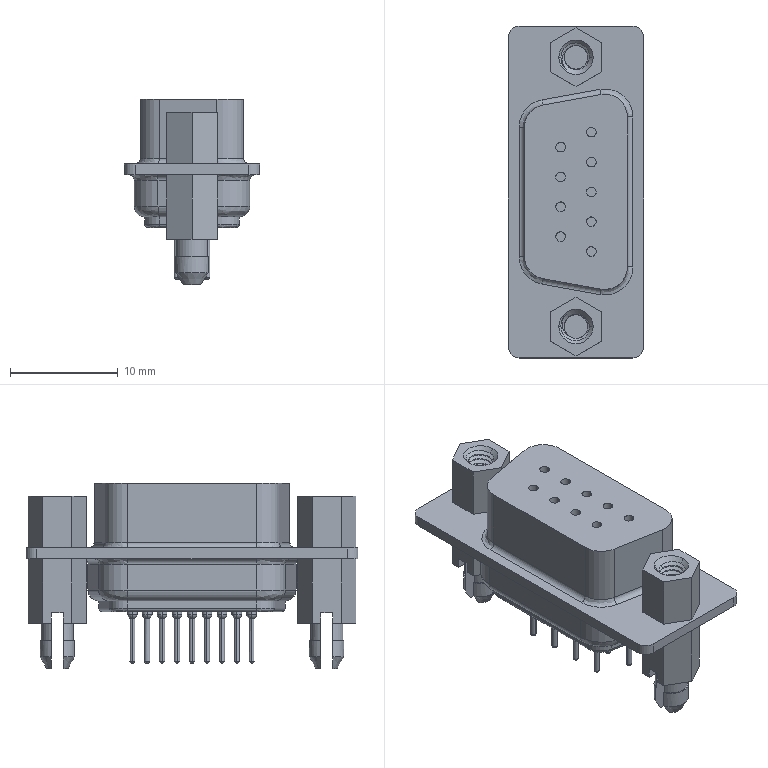Part | SolidWorks | features BaseBody 1 | 1 solid | 293 faces | box 12.55 x 30.81 x 17.2 mm | volume 2595 mm3 | cylinder 132 | plane 86 | torus 36 | spline 29 | cone 10 | commonest cylinder face diameters 2.2 x38 0.9 x36 0.5 x18 1 x8 2 x8 0.6 x4